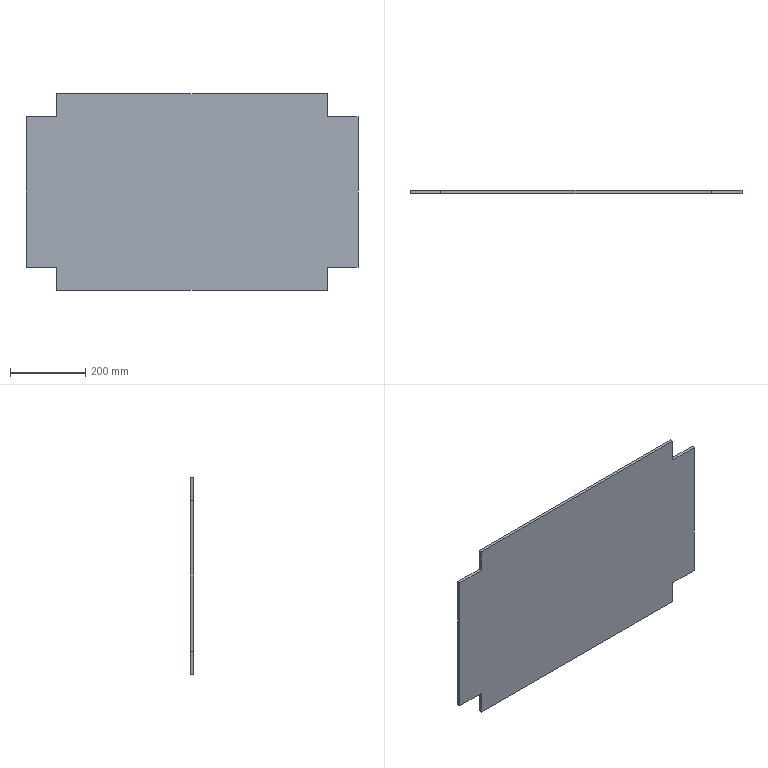Part | STEP file | Guide wheel mechanism revised.sldasm-Part-157 | 1 solid | 14 faces | box 882.42 x 8 x 522.42 mm | volume 3528427 mm3 | plane 14
STEP:
#1=CARTESIAN_POINT('',(-359.9,820.01,-261.21));
#2=VERTEX_POINT('',#1);
#3=CARTESIAN_POINT('',(-359.9,820.01,-199.9));
#4=VERTEX_POINT('',#3);
#5=CARTESIAN_POINT('',(-359.9,820.01,-261.21));
#6=DIRECTION('',(0.,0.,1.));
#7=VECTOR('',#6,1000.);
#8=LINE('',#5,#7);
#9=EDGE_CURVE('',#2,#4,#8,.T.);
#10=ORIENTED_EDGE('',*,*,#9,.T.);
#11=CARTESIAN_POINT('',(-359.9,828.01,-199.9));
#12=VERTEX_POINT('',#11);
#13=CARTESIAN_POINT('',(-359.9,828.01,-199.9));
#14=DIRECTION('',(0.,-1.,0.));
#15=VECTOR('',#14,1000.);
#16=LINE('',#13,#15);
#17=EDGE_CURVE('',#12,#4,#16,.T.);
#18=ORIENTED_EDGE('',*,*,#17,.F.);
#19=CARTESIAN_POINT('',(-359.9,828.01,-261.21));
#20=VERTEX_POINT('',#19);
#21=CARTESIAN_POINT('',(-359.9,828.01,-261.21));
#22=DIRECTION('',(0.,0.,1.));
#23=VECTOR('',#22,1000.);
#24=LINE('',#21,#23);
#25=EDGE_CURVE('',#20,#12,#24,.T.);
#26=ORIENTED_EDGE('',*,*,#25,.F.);
#27=CARTESIAN_POINT('',(-359.9,828.01,-261.21));
#28=DIRECTION('',(0.,-1.,0.));
#29=VECTOR('',#28,1000.);
#30=LINE('',#27,#29);
#31=EDGE_CURVE('',#20,#2,#30,.T.);
#32=ORIENTED_EDGE('',*,*,#31,.T.);
#33=EDGE_LOOP('',(#10,#18,#26,#32));
#34=FACE_OUTER_BOUND('',#33,.T.);
#35=CARTESIAN_POINT('',(-359.9,828.01,-261.21));
#36=DIRECTION('',(1.,0.,0.));
#37=DIRECTION('',(0.,0.,-1.));
#38=AXIS2_PLACEMENT_3D('',#35,#36,#37);
#39=PLANE('',#38);
#40=ADVANCED_FACE('',(#34),#39,.F.);
#41=CARTESIAN_POINT('',(-441.21,820.01,-199.9));
#42=VERTEX_POINT('',#41);
#43=CARTESIAN_POINT('',(-359.9,820.01,-199.9));
#44=DIRECTION('',(-1.,0.,0.));
#45=VECTOR('',#44,1000.);
#46=LINE('',#43,#45);
#47=EDGE_CURVE('',#4,#42,#46,.T.);
#48=ORIENTED_EDGE('',*,*,#47,.T.);
#49=CARTESIAN_POINT('',(-441.21,828.01,-199.9));
#50=VERTEX_POINT('',#49);
#51=CARTESIAN_POINT('',(-441.21,828.01,-199.9));
#52=DIRECTION('',(0.,-1.,0.));
#53=VECTOR('',#52,1000.);
#54=LINE('',#51,#53);
#55=EDGE_CURVE('',#50,#42,#54,.T.);
#56=ORIENTED_EDGE('',*,*,#55,.F.);
#57=CARTESIAN_POINT('',(-359.9,828.01,-199.9));
#58=DIRECTION('',(-1.,0.,0.));
#59=VECTOR('',#58,1000.);
#60=LINE('',#57,#59);
#61=EDGE_CURVE('',#12,#50,#60,.T.);
#62=ORIENTED_EDGE('',*,*,#61,.F.);
#63=ORIENTED_EDGE('',*,*,#17,.T.);
#64=EDGE_LOOP('',(#48,#56,#62,#63));
#65=FACE_OUTER_BOUND('',#64,.T.);
#66=CARTESIAN_POINT('',(-359.9,828.01,-199.9));
#67=DIRECTION('',(0.,0.,1.));
#68=DIRECTION('',(1.,0.,0.));
#69=AXIS2_PLACEMENT_3D('',#66,#67,#68);
#70=PLANE('',#69);
#71=ADVANCED_FACE('',(#65),#70,.F.);
#72=CARTESIAN_POINT('',(-441.21,820.01,199.9));
#73=VERTEX_POINT('',#72);
#74=CARTESIAN_POINT('',(-441.21,820.01,-199.9));
#75=DIRECTION('',(0.,0.,1.));
#76=VECTOR('',#75,1000.);
#77=LINE('',#74,#76);
#78=EDGE_CURVE('',#42,#73,#77,.T.);
#79=ORIENTED_EDGE('',*,*,#78,.T.);
#80=CARTESIAN_POINT('',(-441.21,828.01,199.9));
#81=VERTEX_POINT('',#80);
#82=CARTESIAN_POINT('',(-441.21,828.01,199.9));
#83=DIRECTION('',(0.,-1.,0.));
#84=VECTOR('',#83,1000.);
#85=LINE('',#82,#84);
#86=EDGE_CURVE('',#81,#73,#85,.T.);
#87=ORIENTED_EDGE('',*,*,#86,.F.);
#88=CARTESIAN_POINT('',(-441.21,828.01,-199.9));
#89=DIRECTION('',(0.,0.,1.));
#90=VECTOR('',#89,1000.);
#91=LINE('',#88,#90);
#92=EDGE_CURVE('',#50,#81,#91,.T.);
#93=ORIENTED_EDGE('',*,*,#92,.F.);
#94=ORIENTED_EDGE('',*,*,#55,.T.);
#95=EDGE_LOOP('',(#79,#87,#93,#94));
#96=FACE_OUTER_BOUND('',#95,.T.);
#97=CARTESIAN_POINT('',(-441.21,828.01,-199.9));
#98=DIRECTION('',(1.,0.,0.));
#99=DIRECTION('',(0.,0.,-1.));
#100=AXIS2_PLACEMENT_3D('',#97,#98,#99);
#101=PLANE('',#100);
#102=ADVANCED_FACE('',(#96),#101,.F.);
#103=CARTESIAN_POINT('',(-359.9,820.01,199.9));
#104=VERTEX_POINT('',#103);
#105=CARTESIAN_POINT('',(-441.21,820.01,199.9));
#106=DIRECTION('',(1.,0.,0.));
#107=VECTOR('',#106,1000.);
#108=LINE('',#105,#107);
#109=EDGE_CURVE('',#73,#104,#108,.T.);
#110=ORIENTED_EDGE('',*,*,#109,.T.);
#111=CARTESIAN_POINT('',(-359.9,828.01,199.9));
#112=VERTEX_POINT('',#111);
#113=CARTESIAN_POINT('',(-359.9,828.01,199.9));
#114=DIRECTION('',(0.,-1.,0.));
#115=VECTOR('',#114,1000.);
#116=LINE('',#113,#115);
#117=EDGE_CURVE('',#112,#104,#116,.T.);
#118=ORIENTED_EDGE('',*,*,#117,.F.);
#119=CARTESIAN_POINT('',(-441.21,828.01,199.9));
#120=DIRECTION('',(1.,0.,0.));
#121=VECTOR('',#120,1000.);
#122=LINE('',#119,#121);
#123=EDGE_CURVE('',#81,#112,#122,.T.);
#124=ORIENTED_EDGE('',*,*,#123,.F.);
#125=ORIENTED_EDGE('',*,*,#86,.T.);
#126=EDGE_LOOP('',(#110,#118,#124,#125));
#127=FACE_OUTER_BOUND('',#126,.T.);
#128=CARTESIAN_POINT('',(-441.21,828.01,199.9));
#129=DIRECTION('',(0.,0.,-1.));
#130=DIRECTION('',(-1.,0.,0.));
#131=AXIS2_PLACEMENT_3D('',#128,#129,#130);
#132=PLANE('',#131);
#133=ADVANCED_FACE('',(#127),#132,.F.);
#134=CARTESIAN_POINT('',(-359.9,820.01,261.21));
#135=VERTEX_POINT('',#134);
#136=CARTESIAN_POINT('',(-359.9,820.01,199.9));
#137=DIRECTION('',(0.,0.,1.));
#138=VECTOR('',#137,1000.);
#139=LINE('',#136,#138);
#140=EDGE_CURVE('',#104,#135,#139,.T.);
#141=ORIENTED_EDGE('',*,*,#140,.T.);
#142=CARTESIAN_POINT('',(-359.9,828.01,261.21));
#143=VERTEX_POINT('',#142);
#144=CARTESIAN_POINT('',(-359.9,828.01,261.21));
#145=DIRECTION('',(0.,-1.,0.));
#146=VECTOR('',#145,1000.);
#147=LINE('',#144,#146);
#148=EDGE_CURVE('',#143,#135,#147,.T.);
#149=ORIENTED_EDGE('',*,*,#148,.F.);
#150=CARTESIAN_POINT('',(-359.9,828.01,199.9));
#151=DIRECTION('',(0.,0.,1.));
#152=VECTOR('',#151,1000.);
#153=LINE('',#150,#152);
#154=EDGE_CURVE('',#112,#143,#153,.T.);
#155=ORIENTED_EDGE('',*,*,#154,.F.);
#156=ORIENTED_EDGE('',*,*,#117,.T.);
#157=EDGE_LOOP('',(#141,#149,#155,#156));
#158=FACE_OUTER_BOUND('',#157,.T.);
#159=CARTESIAN_POINT('',(-359.9,828.01,199.9));
#160=DIRECTION('',(1.,0.,0.));
#161=DIRECTION('',(0.,0.,-1.));
#162=AXIS2_PLACEMENT_3D('',#159,#160,#161);
#163=PLANE('',#162);
#164=ADVANCED_FACE('',(#158),#163,.F.);
#165=CARTESIAN_POINT('',(359.9,820.01,261.21));
#166=VERTEX_POINT('',#165);
#167=CARTESIAN_POINT('',(0.,820.01,261.21));
#168=DIRECTION('',(1.,0.,0.));
#169=VECTOR('',#168,1000.);
#170=LINE('',#167,#169);
#171=EDGE_CURVE('',#135,#166,#170,.T.);
#172=ORIENTED_EDGE('',*,*,#171,.T.);
#173=CARTESIAN_POINT('',(359.9,828.01,261.21));
#174=VERTEX_POINT('',#173);
#175=CARTESIAN_POINT('',(359.9,828.01,261.21));
#176=DIRECTION('',(0.,-1.,0.));
#177=VECTOR('',#176,1000.);
#178=LINE('',#175,#177);
#179=EDGE_CURVE('',#174,#166,#178,.T.);
#180=ORIENTED_EDGE('',*,*,#179,.F.);
#181=CARTESIAN_POINT('',(-359.9,828.01,261.21));
#182=DIRECTION('',(1.,0.,0.));
#183=VECTOR('',#182,1000.);
#184=LINE('',#181,#183);
#185=EDGE_CURVE('',#143,#174,#184,.T.);
#186=ORIENTED_EDGE('',*,*,#185,.F.);
#187=ORIENTED_EDGE('',*,*,#148,.T.);
#188=EDGE_LOOP('',(#172,#180,#186,#187));
#189=FACE_OUTER_BOUND('',#188,.T.);
#190=CARTESIAN_POINT('',(0.,828.01,261.21));
#191=DIRECTION('',(0.,0.,-1.));
#192=DIRECTION('',(-1.,0.,0.));
#193=AXIS2_PLACEMENT_3D('',#190,#191,#192);
#194=PLANE('',#193);
#195=ADVANCED_FACE('',(#189),#194,.F.);
#196=CARTESIAN_POINT('',(359.9,820.01,199.9));
#197=VERTEX_POINT('',#196);
#198=CARTESIAN_POINT('',(359.9,820.01,261.21));
#199=DIRECTION('',(0.,0.,-1.));
#200=VECTOR('',#199,1000.);
#201=LINE('',#198,#200);
#202=EDGE_CURVE('',#166,#197,#201,.T.);
#203=ORIENTED_EDGE('',*,*,#202,.T.);
#204=CARTESIAN_POINT('',(359.9,828.01,199.9));
#205=VERTEX_POINT('',#204);
#206=CARTESIAN_POINT('',(359.9,828.01,199.9));
#207=DIRECTION('',(0.,-1.,0.));
#208=VECTOR('',#207,1000.);
#209=LINE('',#206,#208);
#210=EDGE_CURVE('',#205,#197,#209,.T.);
#211=ORIENTED_EDGE('',*,*,#210,.F.);
#212=CARTESIAN_POINT('',(359.9,828.01,261.21));
#213=DIRECTION('',(0.,0.,-1.));
#214=VECTOR('',#213,1000.);
#215=LINE('',#212,#214);
#216=EDGE_CURVE('',#174,#205,#215,.T.);
#217=ORIENTED_EDGE('',*,*,#216,.F.);
#218=ORIENTED_EDGE('',*,*,#179,.T.);
#219=EDGE_LOOP('',(#203,#211,#217,#218));
#220=FACE_OUTER_BOUND('',#219,.T.);
#221=CARTESIAN_POINT('',(359.9,828.01,261.21));
#222=DIRECTION('',(-1.,0.,0.));
#223=DIRECTION('',(0.,0.,1.));
#224=AXIS2_PLACEMENT_3D('',#221,#222,#223);
#225=PLANE('',#224);
#226=ADVANCED_FACE('',(#220),#225,.F.);
#227=CARTESIAN_POINT('',(441.21,820.01,199.9));
#228=VERTEX_POINT('',#227);
#229=CARTESIAN_POINT('',(359.9,820.01,199.9));
#230=DIRECTION('',(1.,0.,0.));
#231=VECTOR('',#230,1000.);
#232=LINE('',#229,#231);
#233=EDGE_CURVE('',#197,#228,#232,.T.);
#234=ORIENTED_EDGE('',*,*,#233,.T.);
#235=CARTESIAN_POINT('',(441.21,828.01,199.9));
#236=VERTEX_POINT('',#235);
#237=CARTESIAN_POINT('',(441.21,828.01,199.9));
#238=DIRECTION('',(0.,-1.,0.));
#239=VECTOR('',#238,1000.);
#240=LINE('',#237,#239);
#241=EDGE_CURVE('',#236,#228,#240,.T.);
#242=ORIENTED_EDGE('',*,*,#241,.F.);
#243=CARTESIAN_POINT('',(359.9,828.01,199.9));
#244=DIRECTION('',(1.,0.,0.));
#245=VECTOR('',#244,1000.);
#246=LINE('',#243,#245);
#247=EDGE_CURVE('',#205,#236,#246,.T.);
#248=ORIENTED_EDGE('',*,*,#247,.F.);
#249=ORIENTED_EDGE('',*,*,#210,.T.);
#250=EDGE_LOOP('',(#234,#242,#248,#249));
#251=FACE_OUTER_BOUND('',#250,.T.);
#252=CARTESIAN_POINT('',(359.9,828.01,199.9));
#253=DIRECTION('',(0.,0.,-1.));
#254=DIRECTION('',(-1.,0.,0.));
#255=AXIS2_PLACEMENT_3D('',#252,#253,#254);
#256=PLANE('',#255);
#257=ADVANCED_FACE('',(#251),#256,.F.);
#258=CARTESIAN_POINT('',(441.21,820.01,-199.9));
#259=VERTEX_POINT('',#258);
#260=CARTESIAN_POINT('',(441.21,820.01,199.9));
#261=DIRECTION('',(0.,0.,-1.));
#262=VECTOR('',#261,1000.);
#263=LINE('',#260,#262);
#264=EDGE_CURVE('',#228,#259,#263,.T.);
#265=ORIENTED_EDGE('',*,*,#264,.T.);
#266=CARTESIAN_POINT('',(441.21,828.01,-199.9));
#267=VERTEX_POINT('',#266);
#268=CARTESIAN_POINT('',(441.21,828.01,-199.9));
#269=DIRECTION('',(0.,-1.,0.));
#270=VECTOR('',#269,1000.);
#271=LINE('',#268,#270);
#272=EDGE_CURVE('',#267,#259,#271,.T.);
#273=ORIENTED_EDGE('',*,*,#272,.F.);
#274=CARTESIAN_POINT('',(441.21,828.01,199.9));
#275=DIRECTION('',(0.,0.,-1.));
#276=VECTOR('',#275,1000.);
#277=LINE('',#274,#276);
#278=EDGE_CURVE('',#236,#267,#277,.T.);
#279=ORIENTED_EDGE('',*,*,#278,.F.);
#280=ORIENTED_EDGE('',*,*,#241,.T.);
#281=EDGE_LOOP('',(#265,#273,#279,#280));
#282=FACE_OUTER_BOUND('',#281,.T.);
#283=CARTESIAN_POINT('',(441.21,828.01,199.9));
#284=DIRECTION('',(-1.,0.,0.));
#285=DIRECTION('',(0.,0.,1.));
#286=AXIS2_PLACEMENT_3D('',#283,#284,#285);
#287=PLANE('',#286);
#288=ADVANCED_FACE('',(#282),#287,.F.);
#289=CARTESIAN_POINT('',(359.9,820.01,-199.9));
#290=VERTEX_POINT('',#289);
#291=CARTESIAN_POINT('',(441.21,820.01,-199.9));
#292=DIRECTION('',(-1.,0.,0.));
#293=VECTOR('',#292,1000.);
#294=LINE('',#291,#293);
#295=EDGE_CURVE('',#259,#290,#294,.T.);
#296=ORIENTED_EDGE('',*,*,#295,.T.);
#297=CARTESIAN_POINT('',(359.9,828.01,-199.9));
#298=VERTEX_POINT('',#297);
#299=CARTESIAN_POINT('',(359.9,828.01,-199.9));
#300=DIRECTION('',(0.,-1.,0.));
#301=VECTOR('',#300,1000.);
#302=LINE('',#299,#301);
#303=EDGE_CURVE('',#298,#290,#302,.T.);
#304=ORIENTED_EDGE('',*,*,#303,.F.);
#305=CARTESIAN_POINT('',(441.21,828.01,-199.9));
#306=DIRECTION('',(-1.,0.,0.));
#307=VECTOR('',#306,1000.);
#308=LINE('',#305,#307);
#309=EDGE_CURVE('',#267,#298,#308,.T.);
#310=ORIENTED_EDGE('',*,*,#309,.F.);
#311=ORIENTED_EDGE('',*,*,#272,.T.);
#312=EDGE_LOOP('',(#296,#304,#310,#311));
#313=FACE_OUTER_BOUND('',#312,.T.);
#314=CARTESIAN_POINT('',(441.21,828.01,-199.9));
#315=DIRECTION('',(0.,0.,1.));
#316=DIRECTION('',(1.,0.,0.));
#317=AXIS2_PLACEMENT_3D('',#314,#315,#316);
#318=PLANE('',#317);
#319=ADVANCED_FACE('',(#313),#318,.F.);
#320=CARTESIAN_POINT('',(359.9,820.01,-261.21));
#321=VERTEX_POINT('',#320);
#322=CARTESIAN_POINT('',(359.9,820.01,-199.9));
#323=DIRECTION('',(0.,0.,-1.));
#324=VECTOR('',#323,1000.);
#325=LINE('',#322,#324);
#326=EDGE_CURVE('',#290,#321,#325,.T.);
#327=ORIENTED_EDGE('',*,*,#326,.T.);
#328=CARTESIAN_POINT('',(359.9,828.01,-261.21));
#329=VERTEX_POINT('',#328);
#330=CARTESIAN_POINT('',(359.9,828.01,-261.21));
#331=DIRECTION('',(0.,-1.,0.));
#332=VECTOR('',#331,1000.);
#333=LINE('',#330,#332);
#334=EDGE_CURVE('',#329,#321,#333,.T.);
#335=ORIENTED_EDGE('',*,*,#334,.F.);
#336=CARTESIAN_POINT('',(359.9,828.01,-199.9));
#337=DIRECTION('',(0.,0.,-1.));
#338=VECTOR('',#337,1000.);
#339=LINE('',#336,#338);
#340=EDGE_CURVE('',#298,#329,#339,.T.);
#341=ORIENTED_EDGE('',*,*,#340,.F.);
#342=ORIENTED_EDGE('',*,*,#303,.T.);
#343=EDGE_LOOP('',(#327,#335,#341,#342));
#344=FACE_OUTER_BOUND('',#343,.T.);
#345=CARTESIAN_POINT('',(359.9,828.01,-199.9));
#346=DIRECTION('',(-1.,0.,0.));
#347=DIRECTION('',(0.,0.,1.));
#348=AXIS2_PLACEMENT_3D('',#345,#346,#347);
#349=PLANE('',#348);
#350=ADVANCED_FACE('',(#344),#349,.F.);
#351=CARTESIAN_POINT('',(0.,820.01,-261.21));
#352=DIRECTION('',(-1.,0.,0.));
#353=VECTOR('',#352,1000.);
#354=LINE('',#351,#353);
#355=EDGE_CURVE('',#321,#2,#354,.T.);
#356=ORIENTED_EDGE('',*,*,#355,.T.);
#357=ORIENTED_EDGE('',*,*,#31,.F.);
#358=CARTESIAN_POINT('',(0.,828.01,-261.21));
#359=DIRECTION('',(-1.,0.,0.));
#360=VECTOR('',#359,1000.);
#361=LINE('',#358,#360);
#362=EDGE_CURVE('',#329,#20,#361,.T.);
#363=ORIENTED_EDGE('',*,*,#362,.F.);
#364=ORIENTED_EDGE('',*,*,#334,.T.);
#365=EDGE_LOOP('',(#356,#357,#363,#364));
#366=FACE_OUTER_BOUND('',#365,.T.);
#367=CARTESIAN_POINT('',(0.,828.01,-261.21));
#368=DIRECTION('',(0.,0.,1.));
#369=DIRECTION('',(1.,0.,0.));
#370=AXIS2_PLACEMENT_3D('',#367,#368,#369);
#371=PLANE('',#370);
#372=ADVANCED_FACE('',(#366),#371,.F.);
#373=ORIENTED_EDGE('',*,*,#216,.T.);
#374=ORIENTED_EDGE('',*,*,#247,.T.);
#375=ORIENTED_EDGE('',*,*,#278,.T.);
#376=ORIENTED_EDGE('',*,*,#309,.T.);
#377=ORIENTED_EDGE('',*,*,#340,.T.);
#378=ORIENTED_EDGE('',*,*,#362,.T.);
#379=ORIENTED_EDGE('',*,*,#25,.T.);
#380=ORIENTED_EDGE('',*,*,#61,.T.);
#381=ORIENTED_EDGE('',*,*,#92,.T.);
#382=ORIENTED_EDGE('',*,*,#123,.T.);
#383=ORIENTED_EDGE('',*,*,#154,.T.);
#384=ORIENTED_EDGE('',*,*,#185,.T.);
#385=EDGE_LOOP('',(#373,#374,#375,#376,#377,#378,#379,#380,#381,#382,#383,#384));
#386=FACE_OUTER_BOUND('',#385,.T.);
#387=CARTESIAN_POINT('',(0.,828.01,0.));
#388=DIRECTION('',(0.,1.,0.));
#389=DIRECTION('',(0.,0.,1.));
#390=AXIS2_PLACEMENT_3D('',#387,#388,#389);
#391=PLANE('',#390);
#392=ADVANCED_FACE('',(#386),#391,.T.);
#393=ORIENTED_EDGE('',*,*,#9,.F.);
#394=ORIENTED_EDGE('',*,*,#355,.F.);
#395=ORIENTED_EDGE('',*,*,#326,.F.);
#396=ORIENTED_EDGE('',*,*,#295,.F.);
#397=ORIENTED_EDGE('',*,*,#264,.F.);
#398=ORIENTED_EDGE('',*,*,#233,.F.);
#399=ORIENTED_EDGE('',*,*,#202,.F.);
#400=ORIENTED_EDGE('',*,*,#171,.F.);
#401=ORIENTED_EDGE('',*,*,#140,.F.);
#402=ORIENTED_EDGE('',*,*,#109,.F.);
#403=ORIENTED_EDGE('',*,*,#78,.F.);
#404=ORIENTED_EDGE('',*,*,#47,.F.);
#405=EDGE_LOOP('',(#393,#394,#395,#396,#397,#398,#399,#400,#401,#402,#403,#404));
#406=FACE_OUTER_BOUND('',#405,.T.);
#407=CARTESIAN_POINT('',(0.,820.01,0.));
#408=DIRECTION('',(0.,1.,0.));
#409=DIRECTION('',(0.,0.,1.));
#410=AXIS2_PLACEMENT_3D('',#407,#408,#409);
#411=PLANE('',#410);
#412=ADVANCED_FACE('',(#406),#411,.F.);
#413=CLOSED_SHELL('',(#40,#71,#102,#133,#164,#195,#226,#257,#288,#319,#350,#372,#392,#412));
#414=MANIFOLD_SOLID_BREP('',#413);
#415=CARTESIAN_POINT('',(0.,0.,0.));
#416=DIRECTION('',(0.,0.,1.));
#417=DIRECTION('',(1.,0.,0.));
#418=AXIS2_PLACEMENT_3D('',#415,#416,#417);
#419=(LENGTH_UNIT()NAMED_UNIT(*)SI_UNIT(.MILLI.,.METRE.));
#420=UNCERTAINTY_MEASURE_WITH_UNIT(LENGTH_MEASURE(0.00001),#419,'','');
#421=(NAMED_UNIT(*)PLANE_ANGLE_UNIT()SI_UNIT($,.RADIAN.));
#422=(NAMED_UNIT(*)SI_UNIT($,.STERADIAN.)SOLID_ANGLE_UNIT());
#423=(GEOMETRIC_REPRESENTATION_CONTEXT(3)GLOBAL_UNCERTAINTY_ASSIGNED_CONTEXT((#420))GLOBAL_UNIT_ASSIGNED_CONTEXT((#419,#421,#422))REPRESENTATION_CONTEXT('',''));
#424=ADVANCED_BREP_SHAPE_REPRESENTATION('',(#414,#418),#423);